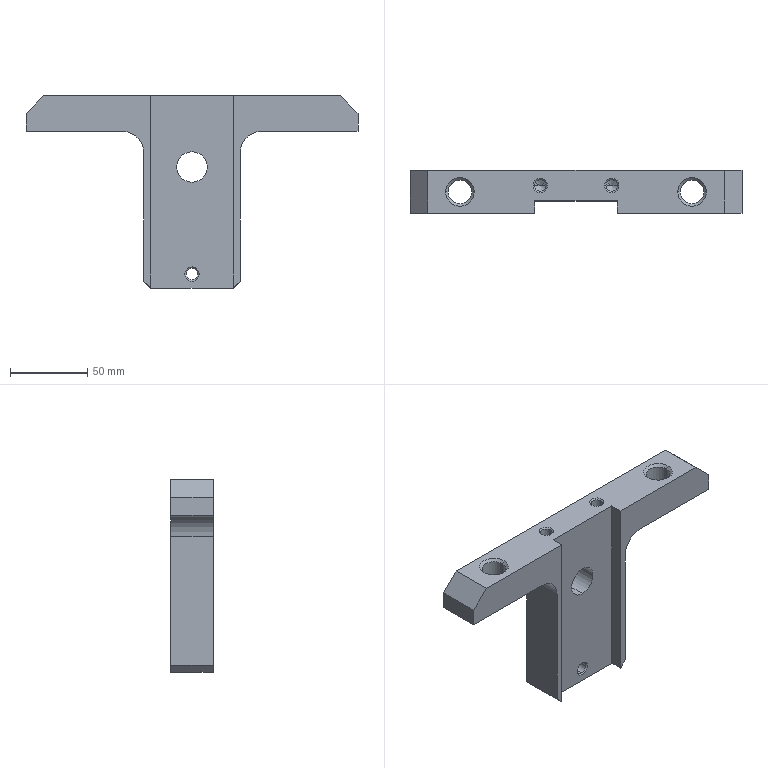Part | SolidWorks | features BaseBody 1 | 1 solid | 55 faces | box 214.615 x 27.692 x 124.615 mm | volume 236727 mm3 | cone 20 | plane 19 | cylinder 16 | commonest cylinder face diameters 7.482 x6 15.339 x4 19.615 x2 27.692 x2 41.538 x2